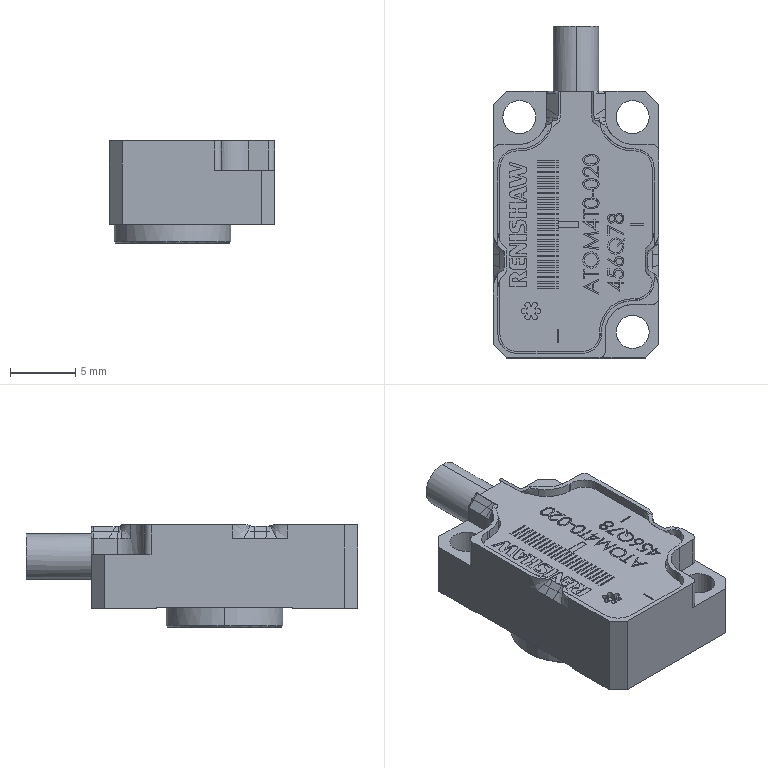Part | STEP file | 2 solids | 614 faces | box 12.7 x 25.5 x 7.883 mm | volume 1498 mm3 | plane 434 | cylinder 105 | spline 73 | cone 2 | commonest cylinder face diameters 0.4 x23 0.1 x10 1.6 x8 2.2 x7 1.1 x6 2.55 x6